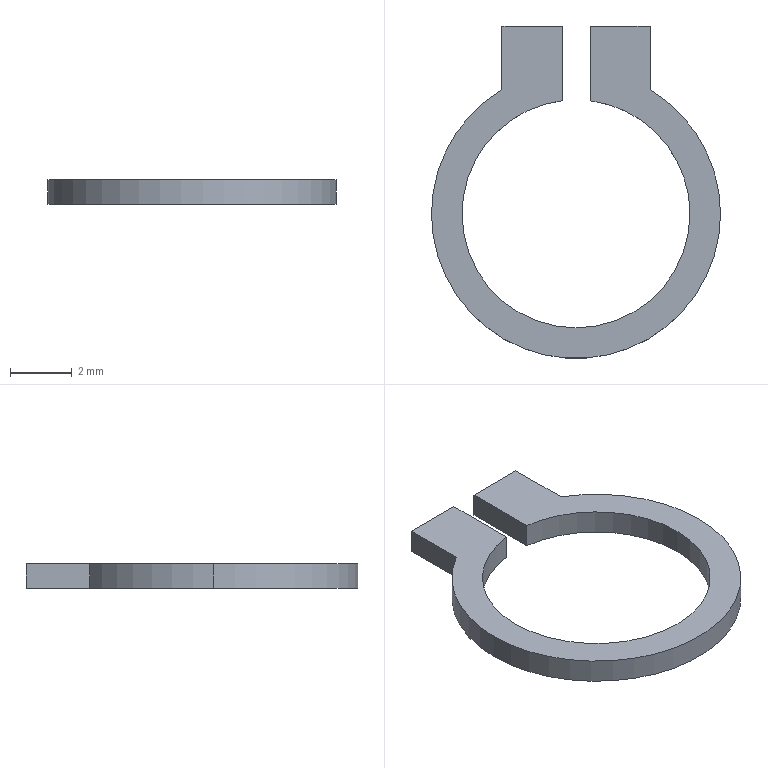Part | SolidWorks | features Extrusion 1 | 1 solid | 14 faces | box 9.38 x 10.788 x 0.8 mm | volume 25.334 mm3 | plane 8 | cylinder 6 | commonest cylinder face diameters 7.4 x3 9.38 x3
STEP:
#1=CARTESIAN_POINT('',(4.69,0.,0.8));
#2=VERTEX_POINT('',#1);
#3=CARTESIAN_POINT('',(2.404,4.027,0.8));
#4=VERTEX_POINT('',#3);
#5=CARTESIAN_POINT('',(0.,0.,0.8));
#6=DIRECTION('',(0.,0.,1.));
#7=DIRECTION('',(1.,0.,0.));
#8=AXIS2_PLACEMENT_3D('',#5,#6,#7);
#9=CIRCLE('',#8,4.69);
#10=EDGE_CURVE('',#2,#4,#9,.T.);
#11=ORIENTED_EDGE('',*,*,#10,.F.);
#12=CARTESIAN_POINT('',(4.69,0.,0.));
#13=VERTEX_POINT('',#12);
#14=CARTESIAN_POINT('',(4.69,0.,0.8));
#15=DIRECTION('',(0.,0.,-1.));
#16=VECTOR('',#15,1000.);
#17=LINE('',#14,#16);
#18=EDGE_CURVE('',#2,#13,#17,.T.);
#19=ORIENTED_EDGE('',*,*,#18,.T.);
#20=CARTESIAN_POINT('',(2.404,4.027,0.));
#21=VERTEX_POINT('',#20);
#22=CARTESIAN_POINT('',(0.,0.,0.));
#23=DIRECTION('',(0.,0.,1.));
#24=DIRECTION('',(1.,0.,0.));
#25=AXIS2_PLACEMENT_3D('',#22,#23,#24);
#26=CIRCLE('',#25,4.69);
#27=EDGE_CURVE('',#13,#21,#26,.T.);
#28=ORIENTED_EDGE('',*,*,#27,.T.);
#29=CARTESIAN_POINT('',(2.404,4.027,0.8));
#30=DIRECTION('',(0.,0.,-1.));
#31=VECTOR('',#30,1000.);
#32=LINE('',#29,#31);
#33=EDGE_CURVE('',#4,#21,#32,.T.);
#34=ORIENTED_EDGE('',*,*,#33,.F.);
#35=EDGE_LOOP('',(#11,#19,#28,#34));
#36=FACE_OUTER_BOUND('',#35,.T.);
#37=CARTESIAN_POINT('',(0.,0.,0.8));
#38=DIRECTION('',(0.,0.,-1.));
#39=DIRECTION('',(-1.,0.,0.));
#40=AXIS2_PLACEMENT_3D('',#37,#38,#39);
#41=CYLINDRICAL_SURFACE('',#40,4.69);
#42=ADVANCED_FACE('',(#36),#41,.T.);
#43=ORIENTED_EDGE('',*,*,#18,.F.);
#44=CARTESIAN_POINT('',(-4.69,0.,0.8));
#45=VERTEX_POINT('',#44);
#46=CARTESIAN_POINT('',(0.,0.,0.8));
#47=DIRECTION('',(0.,0.,1.));
#48=DIRECTION('',(1.,0.,0.));
#49=AXIS2_PLACEMENT_3D('',#46,#47,#48);
#50=CIRCLE('',#49,4.69);
#51=EDGE_CURVE('',#45,#2,#50,.T.);
#52=ORIENTED_EDGE('',*,*,#51,.F.);
#53=CARTESIAN_POINT('',(-4.69,0.,0.));
#54=VERTEX_POINT('',#53);
#55=CARTESIAN_POINT('',(-4.69,0.,0.8));
#56=DIRECTION('',(0.,0.,-1.));
#57=VECTOR('',#56,1000.);
#58=LINE('',#55,#57);
#59=EDGE_CURVE('',#45,#54,#58,.T.);
#60=ORIENTED_EDGE('',*,*,#59,.T.);
#61=CARTESIAN_POINT('',(0.,0.,0.));
#62=DIRECTION('',(0.,0.,1.));
#63=DIRECTION('',(1.,0.,0.));
#64=AXIS2_PLACEMENT_3D('',#61,#62,#63);
#65=CIRCLE('',#64,4.69);
#66=EDGE_CURVE('',#54,#13,#65,.T.);
#67=ORIENTED_EDGE('',*,*,#66,.T.);
#68=EDGE_LOOP('',(#43,#52,#60,#67));
#69=FACE_OUTER_BOUND('',#68,.T.);
#70=CARTESIAN_POINT('',(0.,0.,0.8));
#71=DIRECTION('',(0.,0.,-1.));
#72=DIRECTION('',(-1.,0.,0.));
#73=AXIS2_PLACEMENT_3D('',#70,#71,#72);
#74=CYLINDRICAL_SURFACE('',#73,4.69);
#75=ADVANCED_FACE('',(#69),#74,.T.);
#76=CARTESIAN_POINT('',(3.7,0.,0.8));
#77=VERTEX_POINT('',#76);
#78=CARTESIAN_POINT('',(-3.7,0.,0.8));
#79=VERTEX_POINT('',#78);
#80=CARTESIAN_POINT('',(0.,0.,0.8));
#81=DIRECTION('',(0.,0.,-1.));
#82=DIRECTION('',(1.,0.,0.));
#83=AXIS2_PLACEMENT_3D('',#80,#81,#82);
#84=CIRCLE('',#83,3.7);
#85=EDGE_CURVE('',#77,#79,#84,.T.);
#86=ORIENTED_EDGE('',*,*,#85,.F.);
#87=CARTESIAN_POINT('',(3.7,0.,0.));
#88=VERTEX_POINT('',#87);
#89=CARTESIAN_POINT('',(3.7,0.,0.8));
#90=DIRECTION('',(0.,0.,-1.));
#91=VECTOR('',#90,1000.);
#92=LINE('',#89,#91);
#93=EDGE_CURVE('',#77,#88,#92,.T.);
#94=ORIENTED_EDGE('',*,*,#93,.T.);
#95=CARTESIAN_POINT('',(-3.7,0.,0.));
#96=VERTEX_POINT('',#95);
#97=CARTESIAN_POINT('',(0.,0.,0.));
#98=DIRECTION('',(0.,0.,-1.));
#99=DIRECTION('',(1.,0.,0.));
#100=AXIS2_PLACEMENT_3D('',#97,#98,#99);
#101=CIRCLE('',#100,3.7);
#102=EDGE_CURVE('',#88,#96,#101,.T.);
#103=ORIENTED_EDGE('',*,*,#102,.T.);
#104=CARTESIAN_POINT('',(-3.7,0.,0.8));
#105=DIRECTION('',(0.,0.,-1.));
#106=VECTOR('',#105,1000.);
#107=LINE('',#104,#106);
#108=EDGE_CURVE('',#79,#96,#107,.T.);
#109=ORIENTED_EDGE('',*,*,#108,.F.);
#110=EDGE_LOOP('',(#86,#94,#103,#109));
#111=FACE_OUTER_BOUND('',#110,.T.);
#112=CARTESIAN_POINT('',(0.,0.,0.8));
#113=DIRECTION('',(0.,0.,-1.));
#114=DIRECTION('',(-1.,0.,0.));
#115=AXIS2_PLACEMENT_3D('',#112,#113,#114);
#116=CYLINDRICAL_SURFACE('',#115,3.7);
#117=ADVANCED_FACE('',(#111),#116,.F.);
#118=CARTESIAN_POINT('',(-0.4442,3.673,0.8));
#119=VERTEX_POINT('',#118);
#120=CARTESIAN_POINT('',(0.,0.,0.8));
#121=DIRECTION('',(0.,0.,-1.));
#122=DIRECTION('',(1.,0.,0.));
#123=AXIS2_PLACEMENT_3D('',#120,#121,#122);
#124=CIRCLE('',#123,3.7);
#125=EDGE_CURVE('',#79,#119,#124,.T.);
#126=ORIENTED_EDGE('',*,*,#125,.F.);
#127=ORIENTED_EDGE('',*,*,#108,.T.);
#128=CARTESIAN_POINT('',(-0.4442,3.673,0.));
#129=VERTEX_POINT('',#128);
#130=CARTESIAN_POINT('',(0.,0.,0.));
#131=DIRECTION('',(0.,0.,-1.));
#132=DIRECTION('',(1.,0.,0.));
#133=AXIS2_PLACEMENT_3D('',#130,#131,#132);
#134=CIRCLE('',#133,3.7);
#135=EDGE_CURVE('',#96,#129,#134,.T.);
#136=ORIENTED_EDGE('',*,*,#135,.T.);
#137=CARTESIAN_POINT('',(-0.4442,3.673,0.8));
#138=DIRECTION('',(0.,0.,-1.));
#139=VECTOR('',#138,1000.);
#140=LINE('',#137,#139);
#141=EDGE_CURVE('',#119,#129,#140,.T.);
#142=ORIENTED_EDGE('',*,*,#141,.F.);
#143=EDGE_LOOP('',(#126,#127,#136,#142));
#144=FACE_OUTER_BOUND('',#143,.T.);
#145=CARTESIAN_POINT('',(0.,0.,0.8));
#146=DIRECTION('',(0.,0.,-1.));
#147=DIRECTION('',(-1.,0.,0.));
#148=AXIS2_PLACEMENT_3D('',#145,#146,#147);
#149=CYLINDRICAL_SURFACE('',#148,3.7);
#150=ADVANCED_FACE('',(#144),#149,.F.);
#151=ORIENTED_EDGE('',*,*,#93,.F.);
#152=CARTESIAN_POINT('',(0.4791,3.669,0.8));
#153=VERTEX_POINT('',#152);
#154=CARTESIAN_POINT('',(0.,0.,0.8));
#155=DIRECTION('',(0.,0.,-1.));
#156=DIRECTION('',(1.,0.,0.));
#157=AXIS2_PLACEMENT_3D('',#154,#155,#156);
#158=CIRCLE('',#157,3.7);
#159=EDGE_CURVE('',#153,#77,#158,.T.);
#160=ORIENTED_EDGE('',*,*,#159,.F.);
#161=CARTESIAN_POINT('',(0.4791,3.669,0.));
#162=VERTEX_POINT('',#161);
#163=CARTESIAN_POINT('',(0.4791,3.669,0.8));
#164=DIRECTION('',(0.,0.,-1.));
#165=VECTOR('',#164,1000.);
#166=LINE('',#163,#165);
#167=EDGE_CURVE('',#153,#162,#166,.T.);
#168=ORIENTED_EDGE('',*,*,#167,.T.);
#169=CARTESIAN_POINT('',(0.,0.,0.));
#170=DIRECTION('',(0.,0.,-1.));
#171=DIRECTION('',(1.,0.,0.));
#172=AXIS2_PLACEMENT_3D('',#169,#170,#171);
#173=CIRCLE('',#172,3.7);
#174=EDGE_CURVE('',#162,#88,#173,.T.);
#175=ORIENTED_EDGE('',*,*,#174,.T.);
#176=EDGE_LOOP('',(#151,#160,#168,#175));
#177=FACE_OUTER_BOUND('',#176,.T.);
#178=CARTESIAN_POINT('',(0.,0.,0.8));
#179=DIRECTION('',(0.,0.,-1.));
#180=DIRECTION('',(-1.,0.,0.));
#181=AXIS2_PLACEMENT_3D('',#178,#179,#180);
#182=CYLINDRICAL_SURFACE('',#181,3.7);
#183=ADVANCED_FACE('',(#177),#182,.F.);
#184=CARTESIAN_POINT('',(-0.4442,6.098,0.));
#185=VERTEX_POINT('',#184);
#186=CARTESIAN_POINT('',(-0.4442,3.673,0.));
#187=DIRECTION('',(0.,1.,0.));
#188=VECTOR('',#187,1000.);
#189=LINE('',#186,#188);
#190=EDGE_CURVE('',#129,#185,#189,.T.);
#191=ORIENTED_EDGE('',*,*,#190,.T.);
#192=CARTESIAN_POINT('',(-0.4442,6.098,0.8));
#193=VERTEX_POINT('',#192);
#194=CARTESIAN_POINT('',(-0.4442,6.098,0.8));
#195=DIRECTION('',(0.,0.,-1.));
#196=VECTOR('',#195,1000.);
#197=LINE('',#194,#196);
#198=EDGE_CURVE('',#193,#185,#197,.T.);
#199=ORIENTED_EDGE('',*,*,#198,.F.);
#200=CARTESIAN_POINT('',(-0.4442,3.673,0.8));
#201=DIRECTION('',(0.,1.,0.));
#202=VECTOR('',#201,1000.);
#203=LINE('',#200,#202);
#204=EDGE_CURVE('',#119,#193,#203,.T.);
#205=ORIENTED_EDGE('',*,*,#204,.F.);
#206=ORIENTED_EDGE('',*,*,#141,.T.);
#207=EDGE_LOOP('',(#191,#199,#205,#206));
#208=FACE_OUTER_BOUND('',#207,.T.);
#209=CARTESIAN_POINT('',(-0.4442,3.673,0.8));
#210=DIRECTION('',(-1.,0.,0.));
#211=DIRECTION('',(0.,0.,1.));
#212=AXIS2_PLACEMENT_3D('',#209,#210,#211);
#213=PLANE('',#212);
#214=ADVANCED_FACE('',(#208),#213,.F.);
#215=CARTESIAN_POINT('',(-2.402,6.098,0.));
#216=VERTEX_POINT('',#215);
#217=CARTESIAN_POINT('',(-0.4442,6.098,0.));
#218=DIRECTION('',(-1.,0.,0.));
#219=VECTOR('',#218,1000.);
#220=LINE('',#217,#219);
#221=EDGE_CURVE('',#185,#216,#220,.T.);
#222=ORIENTED_EDGE('',*,*,#221,.T.);
#223=CARTESIAN_POINT('',(-2.402,6.098,0.8));
#224=VERTEX_POINT('',#223);
#225=CARTESIAN_POINT('',(-2.402,6.098,0.8));
#226=DIRECTION('',(0.,0.,-1.));
#227=VECTOR('',#226,1000.);
#228=LINE('',#225,#227);
#229=EDGE_CURVE('',#224,#216,#228,.T.);
#230=ORIENTED_EDGE('',*,*,#229,.F.);
#231=CARTESIAN_POINT('',(-0.4442,6.098,0.8));
#232=DIRECTION('',(-1.,0.,0.));
#233=VECTOR('',#232,1000.);
#234=LINE('',#231,#233);
#235=EDGE_CURVE('',#193,#224,#234,.T.);
#236=ORIENTED_EDGE('',*,*,#235,.F.);
#237=ORIENTED_EDGE('',*,*,#198,.T.);
#238=EDGE_LOOP('',(#222,#230,#236,#237));
#239=FACE_OUTER_BOUND('',#238,.T.);
#240=CARTESIAN_POINT('',(-0.4442,6.098,0.8));
#241=DIRECTION('',(0.,-1.,0.));
#242=DIRECTION('',(0.,0.,-1.));
#243=AXIS2_PLACEMENT_3D('',#240,#241,#242);
#244=PLANE('',#243);
#245=ADVANCED_FACE('',(#239),#244,.F.);
#246=CARTESIAN_POINT('',(-2.402,4.028,0.));
#247=VERTEX_POINT('',#246);
#248=CARTESIAN_POINT('',(-2.402,6.098,0.));
#249=DIRECTION('',(0.,-1.,0.));
#250=VECTOR('',#249,1000.);
#251=LINE('',#248,#250);
#252=EDGE_CURVE('',#216,#247,#251,.T.);
#253=ORIENTED_EDGE('',*,*,#252,.T.);
#254=CARTESIAN_POINT('',(-2.402,4.028,0.8));
#255=VERTEX_POINT('',#254);
#256=CARTESIAN_POINT('',(-2.402,4.028,0.8));
#257=DIRECTION('',(0.,0.,-1.));
#258=VECTOR('',#257,1000.);
#259=LINE('',#256,#258);
#260=EDGE_CURVE('',#255,#247,#259,.T.);
#261=ORIENTED_EDGE('',*,*,#260,.F.);
#262=CARTESIAN_POINT('',(-2.402,6.098,0.8));
#263=DIRECTION('',(0.,-1.,0.));
#264=VECTOR('',#263,1000.);
#265=LINE('',#262,#264);
#266=EDGE_CURVE('',#224,#255,#265,.T.);
#267=ORIENTED_EDGE('',*,*,#266,.F.);
#268=ORIENTED_EDGE('',*,*,#229,.T.);
#269=EDGE_LOOP('',(#253,#261,#267,#268));
#270=FACE_OUTER_BOUND('',#269,.T.);
#271=CARTESIAN_POINT('',(-2.402,6.098,0.8));
#272=DIRECTION('',(1.,0.,0.));
#273=DIRECTION('',(0.,0.,-1.));
#274=AXIS2_PLACEMENT_3D('',#271,#272,#273);
#275=PLANE('',#274);
#276=ADVANCED_FACE('',(#270),#275,.F.);
#277=ORIENTED_EDGE('',*,*,#59,.F.);
#278=CARTESIAN_POINT('',(0.,0.,0.8));
#279=DIRECTION('',(0.,0.,1.));
#280=DIRECTION('',(1.,0.,0.));
#281=AXIS2_PLACEMENT_3D('',#278,#279,#280);
#282=CIRCLE('',#281,4.69);
#283=EDGE_CURVE('',#255,#45,#282,.T.);
#284=ORIENTED_EDGE('',*,*,#283,.F.);
#285=ORIENTED_EDGE('',*,*,#260,.T.);
#286=CARTESIAN_POINT('',(0.,0.,0.));
#287=DIRECTION('',(0.,0.,1.));
#288=DIRECTION('',(1.,0.,0.));
#289=AXIS2_PLACEMENT_3D('',#286,#287,#288);
#290=CIRCLE('',#289,4.69);
#291=EDGE_CURVE('',#247,#54,#290,.T.);
#292=ORIENTED_EDGE('',*,*,#291,.T.);
#293=EDGE_LOOP('',(#277,#284,#285,#292));
#294=FACE_OUTER_BOUND('',#293,.T.);
#295=CARTESIAN_POINT('',(0.,0.,0.8));
#296=DIRECTION('',(0.,0.,-1.));
#297=DIRECTION('',(-1.,0.,0.));
#298=AXIS2_PLACEMENT_3D('',#295,#296,#297);
#299=CYLINDRICAL_SURFACE('',#298,4.69);
#300=ADVANCED_FACE('',(#294),#299,.T.);
#301=CARTESIAN_POINT('',(2.404,6.098,0.));
#302=VERTEX_POINT('',#301);
#303=CARTESIAN_POINT('',(2.404,6.098,0.));
#304=DIRECTION('',(0.,1.,0.));
#305=VECTOR('',#304,1000.);
#306=LINE('',#303,#305);
#307=EDGE_CURVE('',#21,#302,#306,.T.);
#308=ORIENTED_EDGE('',*,*,#307,.T.);
#309=CARTESIAN_POINT('',(2.404,6.098,0.8));
#310=VERTEX_POINT('',#309);
#311=CARTESIAN_POINT('',(2.404,6.098,0.8));
#312=DIRECTION('',(0.,0.,-1.));
#313=VECTOR('',#312,1000.);
#314=LINE('',#311,#313);
#315=EDGE_CURVE('',#310,#302,#314,.T.);
#316=ORIENTED_EDGE('',*,*,#315,.F.);
#317=CARTESIAN_POINT('',(2.404,6.098,0.8));
#318=DIRECTION('',(0.,1.,0.));
#319=VECTOR('',#318,1000.);
#320=LINE('',#317,#319);
#321=EDGE_CURVE('',#4,#310,#320,.T.);
#322=ORIENTED_EDGE('',*,*,#321,.F.);
#323=ORIENTED_EDGE('',*,*,#33,.T.);
#324=EDGE_LOOP('',(#308,#316,#322,#323));
#325=FACE_OUTER_BOUND('',#324,.T.);
#326=CARTESIAN_POINT('',(2.404,6.098,0.8));
#327=DIRECTION('',(-1.,0.,0.));
#328=DIRECTION('',(0.,0.,1.));
#329=AXIS2_PLACEMENT_3D('',#326,#327,#328);
#330=PLANE('',#329);
#331=ADVANCED_FACE('',(#325),#330,.F.);
#332=CARTESIAN_POINT('',(0.4791,6.098,0.));
#333=VERTEX_POINT('',#332);
#334=CARTESIAN_POINT('',(0.4791,6.098,0.));
#335=DIRECTION('',(-1.,0.,0.));
#336=VECTOR('',#335,1000.);
#337=LINE('',#334,#336);
#338=EDGE_CURVE('',#302,#333,#337,.T.);
#339=ORIENTED_EDGE('',*,*,#338,.T.);
#340=CARTESIAN_POINT('',(0.4791,6.098,0.8));
#341=VERTEX_POINT('',#340);
#342=CARTESIAN_POINT('',(0.4791,6.098,0.8));
#343=DIRECTION('',(0.,0.,-1.));
#344=VECTOR('',#343,1000.);
#345=LINE('',#342,#344);
#346=EDGE_CURVE('',#341,#333,#345,.T.);
#347=ORIENTED_EDGE('',*,*,#346,.F.);
#348=CARTESIAN_POINT('',(0.4791,6.098,0.8));
#349=DIRECTION('',(-1.,0.,0.));
#350=VECTOR('',#349,1000.);
#351=LINE('',#348,#350);
#352=EDGE_CURVE('',#310,#341,#351,.T.);
#353=ORIENTED_EDGE('',*,*,#352,.F.);
#354=ORIENTED_EDGE('',*,*,#315,.T.);
#355=EDGE_LOOP('',(#339,#347,#353,#354));
#356=FACE_OUTER_BOUND('',#355,.T.);
#357=CARTESIAN_POINT('',(0.4791,6.098,0.8));
#358=DIRECTION('',(0.,-1.,0.));
#359=DIRECTION('',(0.,0.,-1.));
#360=AXIS2_PLACEMENT_3D('',#357,#358,#359);
#361=PLANE('',#360);
#362=ADVANCED_FACE('',(#356),#361,.F.);
#363=CARTESIAN_POINT('',(0.4791,3.669,0.));
#364=DIRECTION('',(0.,-1.,0.));
#365=VECTOR('',#364,1000.);
#366=LINE('',#363,#365);
#367=EDGE_CURVE('',#333,#162,#366,.T.);
#368=ORIENTED_EDGE('',*,*,#367,.T.);
#369=ORIENTED_EDGE('',*,*,#167,.F.);
#370=CARTESIAN_POINT('',(0.4791,3.669,0.8));
#371=DIRECTION('',(0.,-1.,0.));
#372=VECTOR('',#371,1000.);
#373=LINE('',#370,#372);
#374=EDGE_CURVE('',#341,#153,#373,.T.);
#375=ORIENTED_EDGE('',*,*,#374,.F.);
#376=ORIENTED_EDGE('',*,*,#346,.T.);
#377=EDGE_LOOP('',(#368,#369,#375,#376));
#378=FACE_OUTER_BOUND('',#377,.T.);
#379=CARTESIAN_POINT('',(0.4791,3.669,0.8));
#380=DIRECTION('',(1.,0.,0.));
#381=DIRECTION('',(0.,0.,-1.));
#382=AXIS2_PLACEMENT_3D('',#379,#380,#381);
#383=PLANE('',#382);
#384=ADVANCED_FACE('',(#378),#383,.F.);
#385=ORIENTED_EDGE('',*,*,#159,.T.);
#386=ORIENTED_EDGE('',*,*,#85,.T.);
#387=ORIENTED_EDGE('',*,*,#125,.T.);
#388=ORIENTED_EDGE('',*,*,#204,.T.);
#389=ORIENTED_EDGE('',*,*,#235,.T.);
#390=ORIENTED_EDGE('',*,*,#266,.T.);
#391=ORIENTED_EDGE('',*,*,#283,.T.);
#392=ORIENTED_EDGE('',*,*,#51,.T.);
#393=ORIENTED_EDGE('',*,*,#10,.T.);
#394=ORIENTED_EDGE('',*,*,#321,.T.);
#395=ORIENTED_EDGE('',*,*,#352,.T.);
#396=ORIENTED_EDGE('',*,*,#374,.T.);
#397=EDGE_LOOP('',(#385,#386,#387,#388,#389,#390,#391,#392,#393,#394,#395,#396));
#398=FACE_OUTER_BOUND('',#397,.T.);
#399=CARTESIAN_POINT('',(0.,0.,0.8));
#400=DIRECTION('',(0.,0.,1.));
#401=DIRECTION('',(1.,0.,0.));
#402=AXIS2_PLACEMENT_3D('',#399,#400,#401);
#403=PLANE('',#402);
#404=ADVANCED_FACE('',(#398),#403,.T.);
#405=ORIENTED_EDGE('',*,*,#174,.F.);
#406=ORIENTED_EDGE('',*,*,#367,.F.);
#407=ORIENTED_EDGE('',*,*,#338,.F.);
#408=ORIENTED_EDGE('',*,*,#307,.F.);
#409=ORIENTED_EDGE('',*,*,#27,.F.);
#410=ORIENTED_EDGE('',*,*,#66,.F.);
#411=ORIENTED_EDGE('',*,*,#291,.F.);
#412=ORIENTED_EDGE('',*,*,#252,.F.);
#413=ORIENTED_EDGE('',*,*,#221,.F.);
#414=ORIENTED_EDGE('',*,*,#190,.F.);
#415=ORIENTED_EDGE('',*,*,#135,.F.);
#416=ORIENTED_EDGE('',*,*,#102,.F.);
#417=EDGE_LOOP('',(#405,#406,#407,#408,#409,#410,#411,#412,#413,#414,#415,#416));
#418=FACE_OUTER_BOUND('',#417,.T.);
#419=CARTESIAN_POINT('',(0.,0.,0.));
#420=DIRECTION('',(0.,0.,1.));
#421=DIRECTION('',(1.,0.,0.));
#422=AXIS2_PLACEMENT_3D('',#419,#420,#421);
#423=PLANE('',#422);
#424=ADVANCED_FACE('',(#418),#423,.F.);
#425=CLOSED_SHELL('',(#42,#75,#117,#150,#183,#214,#245,#276,#300,#331,#362,#384,#404,#424));
#426=MANIFOLD_SOLID_BREP('',#425);
#427=CARTESIAN_POINT('',(0.,0.,0.));
#428=DIRECTION('',(0.,0.,1.));
#429=DIRECTION('',(1.,0.,0.));
#430=AXIS2_PLACEMENT_3D('',#427,#428,#429);
#431=(LENGTH_UNIT()NAMED_UNIT(*)SI_UNIT(.MILLI.,.METRE.));
#432=UNCERTAINTY_MEASURE_WITH_UNIT(LENGTH_MEASURE(0.00001),#431,'','');
#433=(NAMED_UNIT(*)PLANE_ANGLE_UNIT()SI_UNIT($,.RADIAN.));
#434=(NAMED_UNIT(*)SI_UNIT($,.STERADIAN.)SOLID_ANGLE_UNIT());
#435=(GEOMETRIC_REPRESENTATION_CONTEXT(3)GLOBAL_UNCERTAINTY_ASSIGNED_CONTEXT((#432))GLOBAL_UNIT_ASSIGNED_CONTEXT((#431,#433,#434))REPRESENTATION_CONTEXT('',''));
#436=ADVANCED_BREP_SHAPE_REPRESENTATION('',(#426,#430),#435);